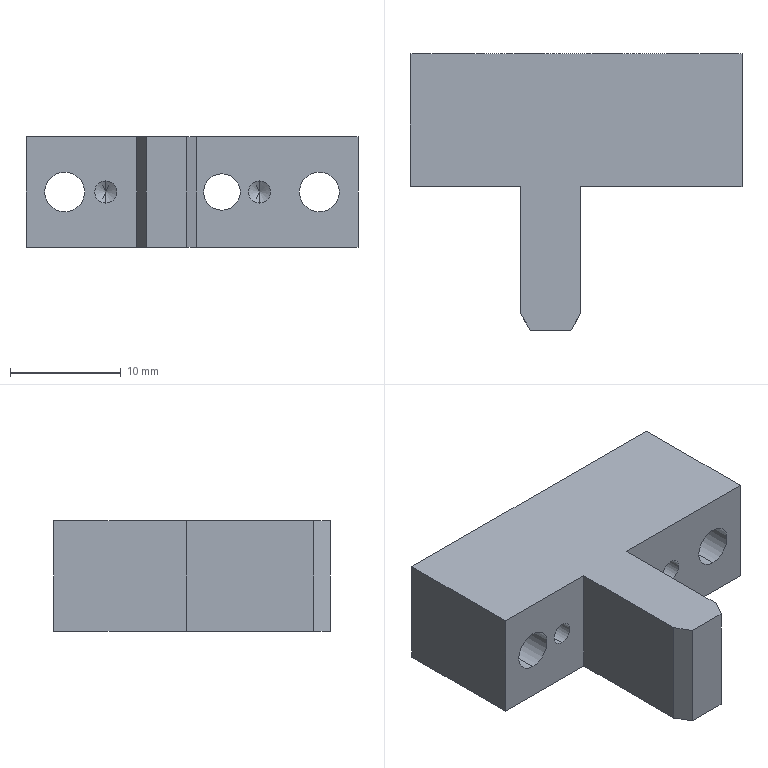Part | STEP file | 22DDSceond144_Default | 1 solid | 36 faces | box 30 x 25 x 10 mm | volume 3740 mm3 | cylinder 16 | plane 14 | cone 6 | commonest cylinder face diameters 2 x4 3.6 x4 6.5 x4 3 x2 3.3 x2